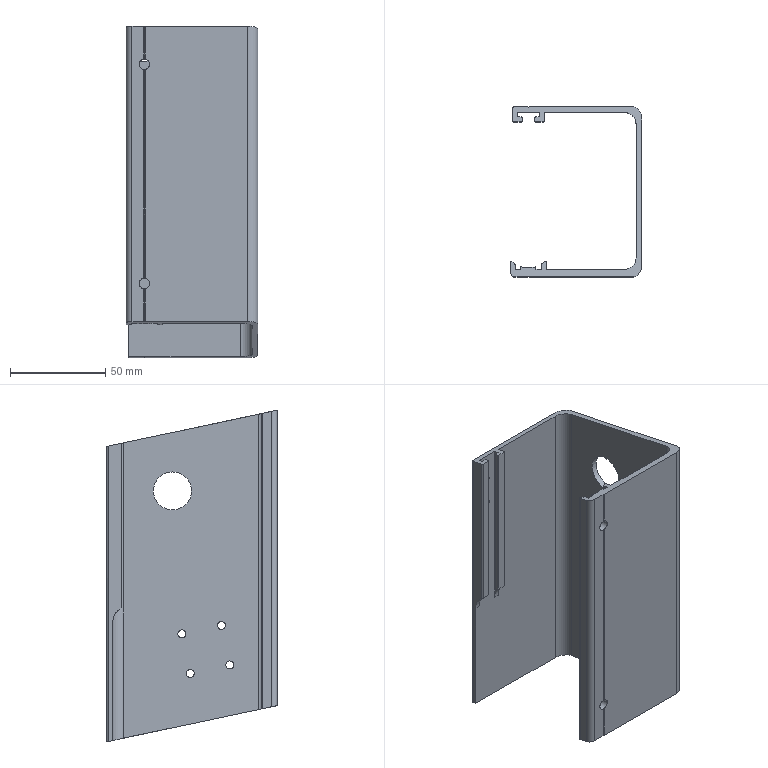Part | STEP file | 31E-01024XJ10 | 1 solid | 81 faces | box 69 x 89.5 x 174.024 mm | volume 118687 mm3 | cylinder 41 | plane 40 | commonest cylinder face diameters 1 x10 4.2 x8 3.2 x4 5.5 x4 20 x4 25.4 x3